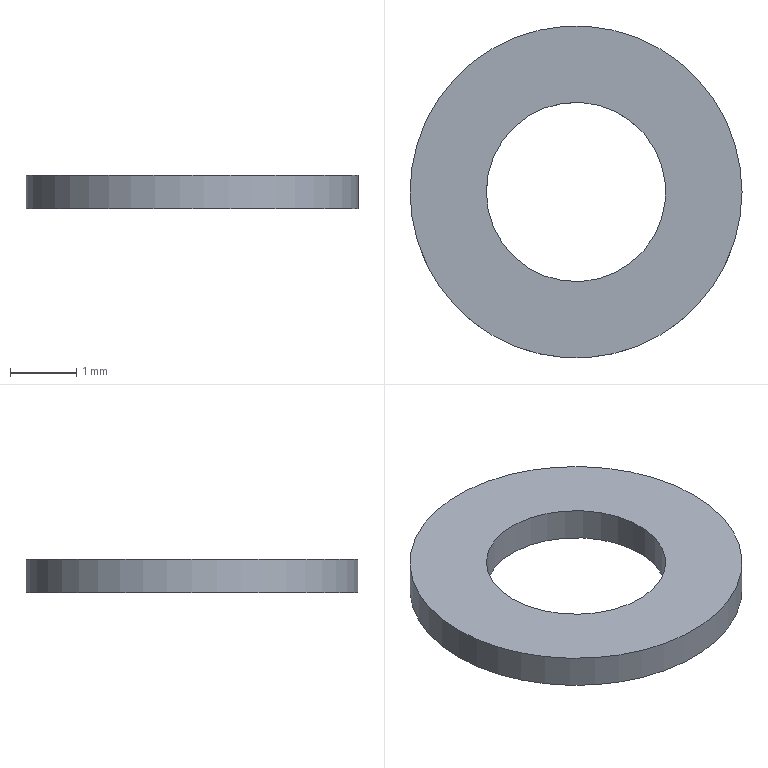Part | STEP file | 1 solid | 4 faces | box 5 x 5 x 0.5 mm | volume 6.955 mm3 | plane 2 | cylinder 2 | commonest cylinder face diameters 2.7 x1 5 x1
STEP:
#1=CARTESIAN_POINT('',(0.,0.,0.));
#2=DIRECTION('',(0.,0.,1.));
#3=DIRECTION('',(1.,0.,0.));
#4=AXIS2_PLACEMENT_3D('',#1,#2,#3);
#5=CARTESIAN_POINT('',(-1.35,0.,-0.25));
#6=VERTEX_POINT('',#5);
#7=CARTESIAN_POINT('',(0.,0.,-0.25));
#8=DIRECTION('',(0.,0.,1.));
#9=DIRECTION('',(-1.,0.,0.));
#10=AXIS2_PLACEMENT_3D('',#7,#8,#9);
#11=CIRCLE('',#10,1.35);
#12=CARTESIAN_POINT('',(0.,0.,-0.25));
#13=DIRECTION('',(0.,0.,-1.));
#14=DIRECTION('',(-1.,0.,0.));
#15=AXIS2_PLACEMENT_3D('',#12,#13,#14);
#16=PLANE('',#15);
#17=CARTESIAN_POINT('',(1.35,0.));
#18=CARTESIAN_POINT('',(1.35,-2.338));
#19=CARTESIAN_POINT('',(-0.675,-1.169));
#20=CARTESIAN_POINT('',(-2.7,0.));
#21=CARTESIAN_POINT('',(-0.675,1.169));
#22=CARTESIAN_POINT('',(1.35,2.338));
#23=CARTESIAN_POINT('',(1.35,0.));
#24=(BOUNDED_CURVE()B_SPLINE_CURVE(2,(#17,#18,#19,#20,#21,#22,#23),.UNSPECIFIED.,.T.,.F.)B_SPLINE_CURVE_WITH_KNOTS((1,2,2,2,2,1),(-2.094,0.,2.094,4.189,6.283,8.378),.UNSPECIFIED.)CURVE()GEOMETRIC_REPRESENTATION_ITEM()RATIONAL_B_SPLINE_CURVE((1.,0.5,1.,0.5,1.,0.5,1.))REPRESENTATION_ITEM(''));
#25=(GEOMETRIC_REPRESENTATION_CONTEXT(2)PARAMETRIC_REPRESENTATION_CONTEXT()REPRESENTATION_CONTEXT('',''));
#26=DEFINITIONAL_REPRESENTATION('',(#24),#25);
#27=PCURVE('',#16,#26);
#28=CARTESIAN_POINT('',(0.,0.,0.275));
#29=DIRECTION('',(0.,0.,-1.));
#30=DIRECTION('',(-1.,0.,0.));
#31=AXIS2_PLACEMENT_3D('',#28,#29,#30);
#32=CYLINDRICAL_SURFACE('',#31,1.35);
#33=CARTESIAN_POINT('',(6.283,0.525));
#34=DIRECTION('',(-1.,0.));
#35=VECTOR('',#34,1.);
#36=LINE('',#33,#35);
#37=(GEOMETRIC_REPRESENTATION_CONTEXT(2)PARAMETRIC_REPRESENTATION_CONTEXT()REPRESENTATION_CONTEXT('',''));
#38=DEFINITIONAL_REPRESENTATION('',(#36),#37);
#39=PCURVE('',#32,#38);
#40=SURFACE_CURVE('',#11,(#27,#39),.PCURVE_S1.);
#41=EDGE_CURVE('',#6,#6,#40,.T.);
#42=ORIENTED_EDGE('',*,*,#41,.T.);
#43=EDGE_LOOP('',(#42));
#44=FACE_BOUND('',#43,.T.);
#45=CARTESIAN_POINT('',(-2.5,0.,-0.25));
#46=VERTEX_POINT('',#45);
#47=CARTESIAN_POINT('',(0.,0.,-0.25));
#48=DIRECTION('',(0.,0.,-1.));
#49=DIRECTION('',(-1.,0.,0.));
#50=AXIS2_PLACEMENT_3D('',#47,#48,#49);
#51=CIRCLE('',#50,2.5);
#52=CARTESIAN_POINT('',(0.,0.));
#53=DIRECTION('',(1.,0.));
#54=AXIS2_PLACEMENT_2D('',#52,#53);
#55=CIRCLE('',#54,2.5);
#56=(GEOMETRIC_REPRESENTATION_CONTEXT(2)PARAMETRIC_REPRESENTATION_CONTEXT()REPRESENTATION_CONTEXT('',''));
#57=DEFINITIONAL_REPRESENTATION('',(#55),#56);
#58=PCURVE('',#16,#57);
#59=CARTESIAN_POINT('',(0.,0.,0.275));
#60=DIRECTION('',(0.,0.,-1.));
#61=DIRECTION('',(-1.,0.,0.));
#62=AXIS2_PLACEMENT_3D('',#59,#60,#61);
#63=CYLINDRICAL_SURFACE('',#62,2.5);
#64=CARTESIAN_POINT('',(0.,0.525));
#65=DIRECTION('',(1.,0.));
#66=VECTOR('',#65,1.);
#67=LINE('',#64,#66);
#68=(GEOMETRIC_REPRESENTATION_CONTEXT(2)PARAMETRIC_REPRESENTATION_CONTEXT()REPRESENTATION_CONTEXT('',''));
#69=DEFINITIONAL_REPRESENTATION('',(#67),#68);
#70=PCURVE('',#63,#69);
#71=SURFACE_CURVE('',#51,(#58,#70),.PCURVE_S1.);
#72=EDGE_CURVE('',#46,#46,#71,.T.);
#73=ORIENTED_EDGE('',*,*,#72,.T.);
#74=EDGE_LOOP('',(#73));
#75=FACE_BOUND('',#74,.T.);
#76=ADVANCED_FACE('',(#44,#75),#16,.T.);
#77=CARTESIAN_POINT('',(-1.35,0.,0.25));
#78=VERTEX_POINT('',#77);
#79=CARTESIAN_POINT('',(0.,0.,0.25));
#80=DIRECTION('',(0.,0.,-1.));
#81=DIRECTION('',(-1.,0.,0.));
#82=AXIS2_PLACEMENT_3D('',#79,#80,#81);
#83=CIRCLE('',#82,1.35);
#84=CARTESIAN_POINT('',(0.,0.025));
#85=DIRECTION('',(1.,0.));
#86=VECTOR('',#85,1.);
#87=LINE('',#84,#86);
#88=(GEOMETRIC_REPRESENTATION_CONTEXT(2)PARAMETRIC_REPRESENTATION_CONTEXT()REPRESENTATION_CONTEXT('',''));
#89=DEFINITIONAL_REPRESENTATION('',(#87),#88);
#90=PCURVE('',#32,#89);
#91=CARTESIAN_POINT('',(0.,0.,0.25));
#92=DIRECTION('',(0.,0.,-1.));
#93=DIRECTION('',(-1.,0.,0.));
#94=AXIS2_PLACEMENT_3D('',#91,#92,#93);
#95=PLANE('',#94);
#96=CARTESIAN_POINT('',(0.,0.));
#97=DIRECTION('',(1.,0.));
#98=AXIS2_PLACEMENT_2D('',#96,#97);
#99=CIRCLE('',#98,1.35);
#100=(GEOMETRIC_REPRESENTATION_CONTEXT(2)PARAMETRIC_REPRESENTATION_CONTEXT()REPRESENTATION_CONTEXT('',''));
#101=DEFINITIONAL_REPRESENTATION('',(#99),#100);
#102=PCURVE('',#95,#101);
#103=SURFACE_CURVE('',#83,(#90,#102),.PCURVE_S1.);
#104=EDGE_CURVE('',#78,#78,#103,.T.);
#105=ORIENTED_EDGE('',*,*,#104,.T.);
#106=CARTESIAN_POINT('',(-1.35,0.,0.25));
#107=CARTESIAN_POINT('',(-1.35,0.,-0.25));
#108=B_SPLINE_CURVE_WITH_KNOTS('',1,(#106,#107),.UNSPECIFIED.,.F.,.F.,(2,2),(0.025,0.525),.PIECEWISE_BEZIER_KNOTS.);
#109=CARTESIAN_POINT('',(6.283,0.));
#110=DIRECTION('',(0.,1.));
#111=VECTOR('',#110,1.);
#112=LINE('',#109,#111);
#113=(GEOMETRIC_REPRESENTATION_CONTEXT(2)PARAMETRIC_REPRESENTATION_CONTEXT()REPRESENTATION_CONTEXT('',''));
#114=DEFINITIONAL_REPRESENTATION('',(#112),#113);
#115=PCURVE('',#32,#114);
#116=CARTESIAN_POINT('',(0.,0.));
#117=DIRECTION('',(0.,1.));
#118=VECTOR('',#117,1.);
#119=LINE('',#116,#118);
#120=(GEOMETRIC_REPRESENTATION_CONTEXT(2)PARAMETRIC_REPRESENTATION_CONTEXT()REPRESENTATION_CONTEXT('',''));
#121=DEFINITIONAL_REPRESENTATION('',(#119),#120);
#122=PCURVE('',#32,#121);
#123=SEAM_CURVE('',#108,(#115,#122),.PCURVE_S1.);
#124=EDGE_CURVE('',#78,#6,#123,.T.);
#125=ORIENTED_EDGE('',*,*,#124,.T.);
#126=ORIENTED_EDGE('',*,*,#41,.T.);
#127=ORIENTED_EDGE('',*,*,#124,.F.);
#128=EDGE_LOOP('',(#105,#125,#126,#127));
#129=FACE_BOUND('',#128,.F.);
#130=ADVANCED_FACE('',(#129),#32,.F.);
#131=ORIENTED_EDGE('',*,*,#72,.F.);
#132=CARTESIAN_POINT('',(-2.5,0.,0.25));
#133=VERTEX_POINT('',#132);
#134=CARTESIAN_POINT('',(-2.5,0.,0.25));
#135=CARTESIAN_POINT('',(-2.5,0.,-0.25));
#136=B_SPLINE_CURVE_WITH_KNOTS('',1,(#134,#135),.UNSPECIFIED.,.F.,.F.,(2,2),(0.025,0.525),.PIECEWISE_BEZIER_KNOTS.);
#137=CARTESIAN_POINT('',(0.,0.));
#138=DIRECTION('',(0.,1.));
#139=VECTOR('',#138,1.);
#140=LINE('',#137,#139);
#141=(GEOMETRIC_REPRESENTATION_CONTEXT(2)PARAMETRIC_REPRESENTATION_CONTEXT()REPRESENTATION_CONTEXT('',''));
#142=DEFINITIONAL_REPRESENTATION('',(#140),#141);
#143=PCURVE('',#63,#142);
#144=CARTESIAN_POINT('',(6.283,0.));
#145=DIRECTION('',(0.,1.));
#146=VECTOR('',#145,1.);
#147=LINE('',#144,#146);
#148=(GEOMETRIC_REPRESENTATION_CONTEXT(2)PARAMETRIC_REPRESENTATION_CONTEXT()REPRESENTATION_CONTEXT('',''));
#149=DEFINITIONAL_REPRESENTATION('',(#147),#148);
#150=PCURVE('',#63,#149);
#151=SEAM_CURVE('',#136,(#143,#150),.PCURVE_S1.);
#152=EDGE_CURVE('',#133,#46,#151,.T.);
#153=ORIENTED_EDGE('',*,*,#152,.F.);
#154=CARTESIAN_POINT('',(0.,0.,0.25));
#155=DIRECTION('',(0.,0.,-1.));
#156=DIRECTION('',(-1.,0.,0.));
#157=AXIS2_PLACEMENT_3D('',#154,#155,#156);
#158=CIRCLE('',#157,2.5);
#159=CARTESIAN_POINT('',(0.,0.025));
#160=DIRECTION('',(1.,0.));
#161=VECTOR('',#160,1.);
#162=LINE('',#159,#161);
#163=(GEOMETRIC_REPRESENTATION_CONTEXT(2)PARAMETRIC_REPRESENTATION_CONTEXT()REPRESENTATION_CONTEXT('',''));
#164=DEFINITIONAL_REPRESENTATION('',(#162),#163);
#165=PCURVE('',#63,#164);
#166=CARTESIAN_POINT('',(0.,0.));
#167=DIRECTION('',(1.,0.));
#168=AXIS2_PLACEMENT_2D('',#166,#167);
#169=CIRCLE('',#168,2.5);
#170=(GEOMETRIC_REPRESENTATION_CONTEXT(2)PARAMETRIC_REPRESENTATION_CONTEXT()REPRESENTATION_CONTEXT('',''));
#171=DEFINITIONAL_REPRESENTATION('',(#169),#170);
#172=PCURVE('',#95,#171);
#173=SURFACE_CURVE('',#158,(#165,#172),.PCURVE_S1.);
#174=EDGE_CURVE('',#133,#133,#173,.T.);
#175=ORIENTED_EDGE('',*,*,#174,.T.);
#176=ORIENTED_EDGE('',*,*,#152,.T.);
#177=EDGE_LOOP('',(#131,#153,#175,#176));
#178=FACE_BOUND('',#177,.T.);
#179=ADVANCED_FACE('',(#178),#63,.T.);
#180=ORIENTED_EDGE('',*,*,#104,.T.);
#181=EDGE_LOOP('',(#180));
#182=FACE_BOUND('',#181,.T.);
#183=ORIENTED_EDGE('',*,*,#174,.F.);
#184=EDGE_LOOP('',(#183));
#185=FACE_BOUND('',#184,.T.);
#186=ADVANCED_FACE('',(#182,#185),#95,.F.);
#187=CLOSED_SHELL('',(#76,#130,#179,#186));
#188=MANIFOLD_SOLID_BREP('',#187);
#189=(LENGTH_UNIT()NAMED_UNIT(*)SI_UNIT(.MILLI.,.METRE.));
#190=UNCERTAINTY_MEASURE_WITH_UNIT(LENGTH_MEASURE(0.00001),#189,'','');
#191=(NAMED_UNIT(*)PLANE_ANGLE_UNIT()SI_UNIT($,.RADIAN.));
#192=(NAMED_UNIT(*)SI_UNIT($,.STERADIAN.)SOLID_ANGLE_UNIT());
#193=(GEOMETRIC_REPRESENTATION_CONTEXT(3)GLOBAL_UNCERTAINTY_ASSIGNED_CONTEXT((#190))GLOBAL_UNIT_ASSIGNED_CONTEXT((#189,#191,#192))REPRESENTATION_CONTEXT('',''));
#194=ADVANCED_BREP_SHAPE_REPRESENTATION('',(#4,#188),#193);